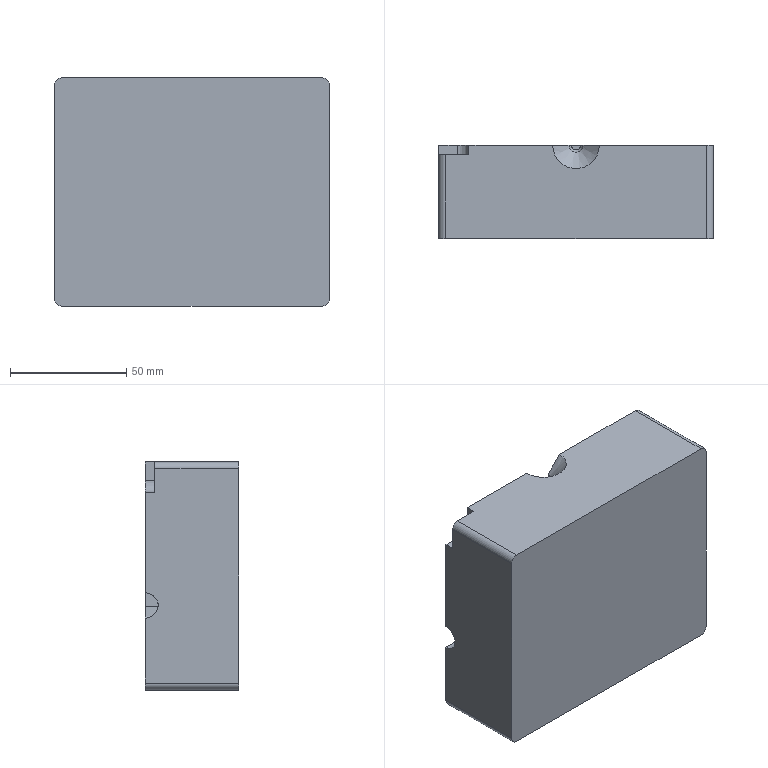CAM job | NX | 3-axis milling | part box 118 x 40 x 98 mm | stock box 118 x 40 x 98 mm
Tools:
number,name,description,diameter,corner_radius,flute_length,length,flutes
0,D8,Milling Tool-5 Parameters,8.0,0.0,50.0,75.0,2
0,D4,Milling Tool-5 Parameters,4.0,0.0,50.0,75.0,2
0,B4,Milling Tool-Ball Mill,4.0,2.0,50.0,75.0,2
0,D8R1,Milling Tool-5 Parameters,8.0,0.0,50.0,75.0,2
0,D4R1,Milling Tool-5 Parameters,4.0,1.0,50.0,75.0,2
Operations:
program,operation,operation_type,tool,method,geometry_group,spindle_rpm,surface_speed,feed_per_tooth,feed_cut,feed_plunge,cut_length_mm,path_length_mm,cut_time_min,machine_time_min
PROGRAM,CAVITY_MILL,CavityMilling,D8,METHOD,WORKPIECE,0.0,0.0,0.0,250.0,100.0,10413.716,11985.158,41.655,41.812
PROGRAM,CAVITY_MILL_COPY,CavityMilling,D4,METHOD,WORKPIECE,0.0,0.0,0.0,250.0,100.0,2529.216,6121.175,10.117,10.476
PROGRAM,FACE_MILLING,FaceMilling,D8,METHOD,WORKPIECE,0.0,0.0,0.0,250.0,100.0,186.515,823.935,0.7461,0.8098
PROGRAM,CONTOUR_AREA,SurfaceContour,B4,METHOD,MCS_MILL,0.0,0.0,0.0,250.0,100.0,19591.302,19772.251,78.365,78.383
PROGRAM,CONTOUR_AREA_COPY,SurfaceContour,B4,METHOD,WORKPIECE,0.0,0.0,0.0,250.0,100.0,3115.895,3258.101,12.464,12.478
PROGRAM,ZLEVEL_PROFILE,ZLevelMilling,D8R1,METHOD,MCS_MILL,0.0,0.0,0.0,250.0,100.0,2793.51,3006.816,11.174,11.195
PROGRAM,CONTOUR_AREA_COPY_COPY,SurfaceContour,B4,METHOD,MCS_MILL,0.0,0.0,0.0,250.0,100.0,953.231,1019.631,3.813,3.82
PROGRAM,ZLEVEL_PROFILE_COPY,ZLevelMilling,D4R1,METHOD,MCS_MILL,0.0,0.0,0.0,250.0,100.0,11522.647,12525.143,46.091,46.191